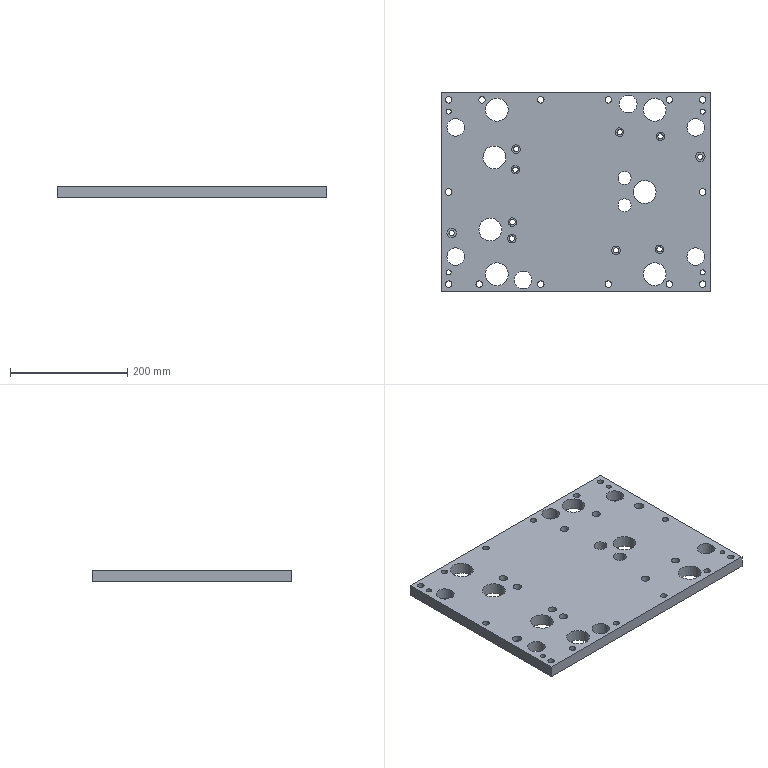Part | NX | features LIN_SOLID_COLOR 2 | 1 solid | 69 faces | box 460 x 340 x 20 mm | volume 2805175 mm3 | cylinder 53 | plane 16 | commonest cylinder face diameters 11 x14 9 x10 14.5 x8 39 x7 30 x6 8.5 x4